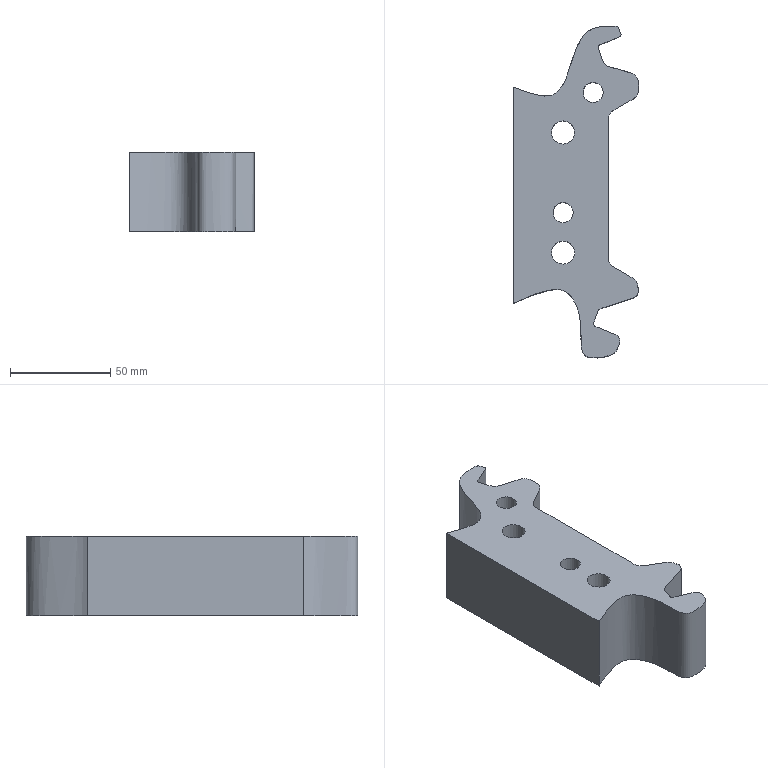Part | NX | features solid 2 | 1 solid | 12 faces | box 62.912 x 165.84 x 39.5 mm | volume 66309 mm3 | cylinder 6 | plane 4 | spline 2 | commonest cylinder face diameters 10 x2 11.5 x2 17.5 x2